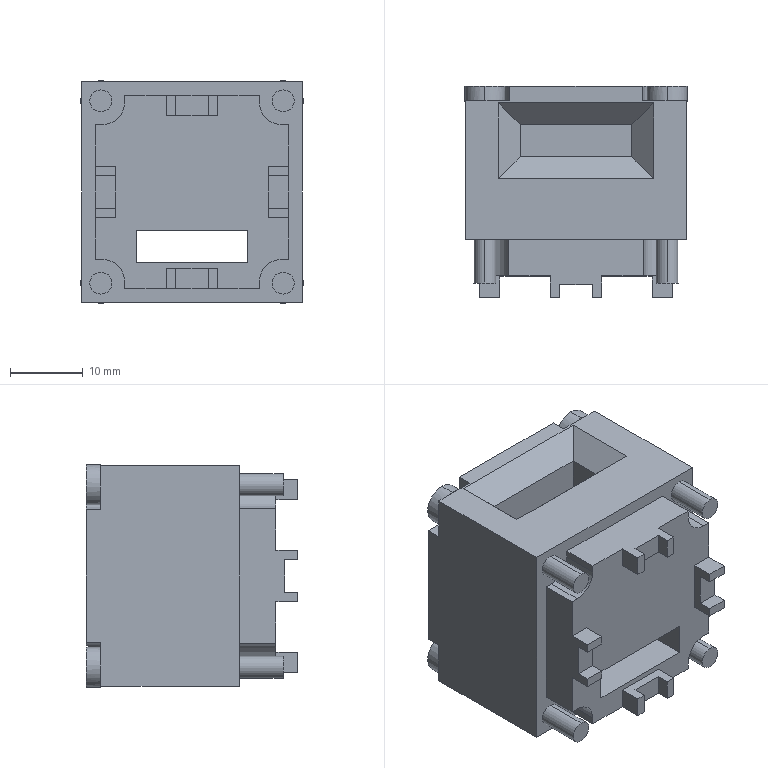Part | STEP file | D4NS_1CF_HEAD^D4NS_1CF_Laser guard | 1 solid | 123 faces | box 30.5 x 29 x 30.5 mm | volume 19068 mm3 | plane 99 | cylinder 24 | commonest cylinder face diameters 3 x8 5.5 x8 6 x8